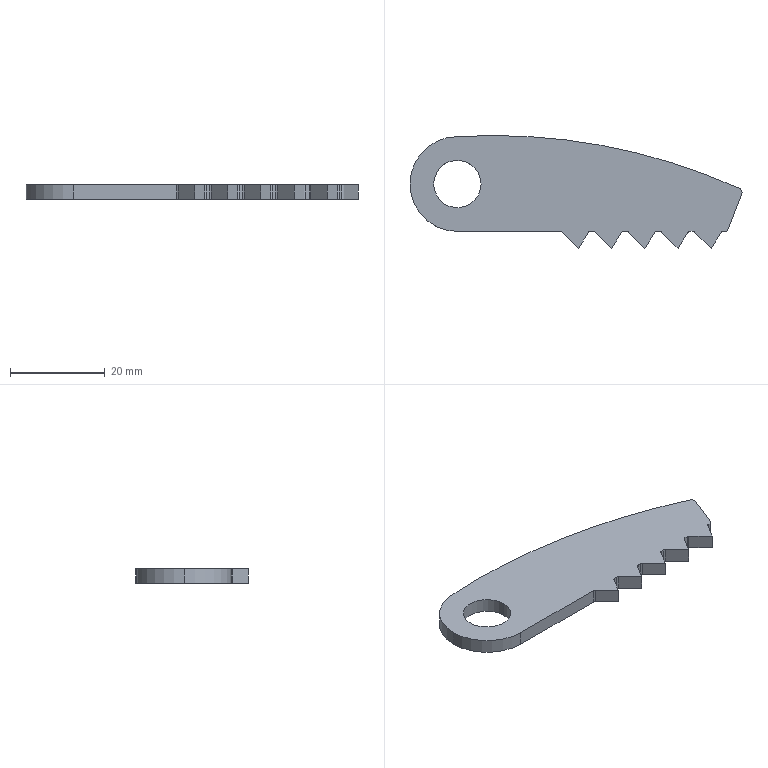Part | SolidWorks | features Extrusion 1, ICE 1 | 1 solid | 36 faces | box 70.059 x 23.839 x 3 mm | volume 3412 mm3 | plane 19 | cylinder 17 | commonest cylinder face diameters 1 x11 10 x2 20 x2 2 x1 252.737 x1
STEP:
#1=CARTESIAN_POINT('',(-5.,0.,0.));
#2=VERTEX_POINT('',#1);
#3=CARTESIAN_POINT('',(5.,0.,0.));
#4=VERTEX_POINT('',#3);
#5=CARTESIAN_POINT('',(0.,0.,0.));
#6=DIRECTION('',(0.,0.,1.));
#7=DIRECTION('',(1.,0.,0.));
#8=AXIS2_PLACEMENT_3D('',#5,#6,#7);
#9=CIRCLE('',#8,5.);
#10=EDGE_CURVE('',#2,#4,#9,.T.);
#11=ORIENTED_EDGE('',*,*,#10,.F.);
#12=CARTESIAN_POINT('',(-5.,0.,3.));
#13=VERTEX_POINT('',#12);
#14=CARTESIAN_POINT('',(-5.,0.,0.));
#15=DIRECTION('',(0.,0.,1.));
#16=VECTOR('',#15,1000.);
#17=LINE('',#14,#16);
#18=EDGE_CURVE('',#2,#13,#17,.T.);
#19=ORIENTED_EDGE('',*,*,#18,.T.);
#20=CARTESIAN_POINT('',(5.,0.,3.));
#21=VERTEX_POINT('',#20);
#22=CARTESIAN_POINT('',(0.,0.,3.));
#23=DIRECTION('',(0.,0.,1.));
#24=DIRECTION('',(1.,0.,0.));
#25=AXIS2_PLACEMENT_3D('',#22,#23,#24);
#26=CIRCLE('',#25,5.);
#27=EDGE_CURVE('',#13,#21,#26,.T.);
#28=ORIENTED_EDGE('',*,*,#27,.T.);
#29=CARTESIAN_POINT('',(5.,0.,0.));
#30=DIRECTION('',(0.,0.,1.));
#31=VECTOR('',#30,1000.);
#32=LINE('',#29,#31);
#33=EDGE_CURVE('',#4,#21,#32,.T.);
#34=ORIENTED_EDGE('',*,*,#33,.F.);
#35=EDGE_LOOP('',(#11,#19,#28,#34));
#36=FACE_OUTER_BOUND('',#35,.T.);
#37=CARTESIAN_POINT('',(0.,0.,0.));
#38=DIRECTION('',(0.,0.,1.));
#39=DIRECTION('',(1.,0.,0.));
#40=AXIS2_PLACEMENT_3D('',#37,#38,#39);
#41=CYLINDRICAL_SURFACE('',#40,5.);
#42=ADVANCED_FACE('',(#36),#41,.F.);
#43=CARTESIAN_POINT('',(-10.,0.,3.));
#44=VERTEX_POINT('',#43);
#45=CARTESIAN_POINT('',(0.,-10.,3.));
#46=VERTEX_POINT('',#45);
#47=CARTESIAN_POINT('',(0.,0.,3.));
#48=DIRECTION('',(0.,0.,1.));
#49=DIRECTION('',(1.,0.,0.));
#50=AXIS2_PLACEMENT_3D('',#47,#48,#49);
#51=CIRCLE('',#50,10.);
#52=EDGE_CURVE('',#44,#46,#51,.T.);
#53=ORIENTED_EDGE('',*,*,#52,.F.);
#54=CARTESIAN_POINT('',(-10.,0.,0.));
#55=VERTEX_POINT('',#54);
#56=CARTESIAN_POINT('',(-10.,0.,3.));
#57=DIRECTION('',(0.,0.,-1.));
#58=VECTOR('',#57,1000.);
#59=LINE('',#56,#58);
#60=EDGE_CURVE('',#44,#55,#59,.T.);
#61=ORIENTED_EDGE('',*,*,#60,.T.);
#62=CARTESIAN_POINT('',(0.,-10.,0.));
#63=VERTEX_POINT('',#62);
#64=CARTESIAN_POINT('',(0.,0.,0.));
#65=DIRECTION('',(0.,0.,1.));
#66=DIRECTION('',(1.,0.,0.));
#67=AXIS2_PLACEMENT_3D('',#64,#65,#66);
#68=CIRCLE('',#67,10.);
#69=EDGE_CURVE('',#55,#63,#68,.T.);
#70=ORIENTED_EDGE('',*,*,#69,.T.);
#71=CARTESIAN_POINT('',(0.,-10.,3.));
#72=DIRECTION('',(0.,0.,-1.));
#73=VECTOR('',#72,1000.);
#74=LINE('',#71,#73);
#75=EDGE_CURVE('',#46,#63,#74,.T.);
#76=ORIENTED_EDGE('',*,*,#75,.F.);
#77=EDGE_LOOP('',(#53,#61,#70,#76));
#78=FACE_OUTER_BOUND('',#77,.T.);
#79=CARTESIAN_POINT('',(0.,0.,3.));
#80=DIRECTION('',(0.,0.,-1.));
#81=DIRECTION('',(-1.,0.,0.));
#82=AXIS2_PLACEMENT_3D('',#79,#80,#81);
#83=CYLINDRICAL_SURFACE('',#82,10.);
#84=ADVANCED_FACE('',(#78),#83,.T.);
#85=ORIENTED_EDGE('',*,*,#60,.F.);
#86=CARTESIAN_POINT('',(-0.189,9.998,3.));
#87=VERTEX_POINT('',#86);
#88=CARTESIAN_POINT('',(0.,0.,3.));
#89=DIRECTION('',(0.,0.,1.));
#90=DIRECTION('',(1.,0.,0.));
#91=AXIS2_PLACEMENT_3D('',#88,#89,#90);
#92=CIRCLE('',#91,10.);
#93=EDGE_CURVE('',#87,#44,#92,.T.);
#94=ORIENTED_EDGE('',*,*,#93,.F.);
#95=CARTESIAN_POINT('',(-0.189,9.998,0.));
#96=VERTEX_POINT('',#95);
#97=CARTESIAN_POINT('',(-0.189,9.998,3.));
#98=DIRECTION('',(0.,0.,-1.));
#99=VECTOR('',#98,1000.);
#100=LINE('',#97,#99);
#101=EDGE_CURVE('',#87,#96,#100,.T.);
#102=ORIENTED_EDGE('',*,*,#101,.T.);
#103=CARTESIAN_POINT('',(0.,0.,0.));
#104=DIRECTION('',(0.,0.,1.));
#105=DIRECTION('',(1.,0.,0.));
#106=AXIS2_PLACEMENT_3D('',#103,#104,#105);
#107=CIRCLE('',#106,10.);
#108=EDGE_CURVE('',#96,#55,#107,.T.);
#109=ORIENTED_EDGE('',*,*,#108,.T.);
#110=EDGE_LOOP('',(#85,#94,#102,#109));
#111=FACE_OUTER_BOUND('',#110,.T.);
#112=CARTESIAN_POINT('',(0.,0.,3.));
#113=DIRECTION('',(0.,0.,-1.));
#114=DIRECTION('',(-1.,0.,0.));
#115=AXIS2_PLACEMENT_3D('',#112,#113,#114);
#116=CYLINDRICAL_SURFACE('',#115,10.);
#117=ADVANCED_FACE('',(#111),#116,.T.);
#118=CARTESIAN_POINT('',(21.748,-10.,0.));
#119=VERTEX_POINT('',#118);
#120=CARTESIAN_POINT('',(0.,-10.,0.));
#121=DIRECTION('',(1.,0.,0.));
#122=VECTOR('',#121,1000.);
#123=LINE('',#120,#122);
#124=EDGE_CURVE('',#63,#119,#123,.T.);
#125=ORIENTED_EDGE('',*,*,#124,.T.);
#126=CARTESIAN_POINT('',(21.748,-10.,3.));
#127=VERTEX_POINT('',#126);
#128=CARTESIAN_POINT('',(21.748,-10.,3.));
#129=DIRECTION('',(0.,0.,-1.));
#130=VECTOR('',#129,1000.);
#131=LINE('',#128,#130);
#132=EDGE_CURVE('',#127,#119,#131,.T.);
#133=ORIENTED_EDGE('',*,*,#132,.F.);
#134=CARTESIAN_POINT('',(0.,-10.,3.));
#135=DIRECTION('',(1.,0.,0.));
#136=VECTOR('',#135,1000.);
#137=LINE('',#134,#136);
#138=EDGE_CURVE('',#46,#127,#137,.T.);
#139=ORIENTED_EDGE('',*,*,#138,.F.);
#140=ORIENTED_EDGE('',*,*,#75,.T.);
#141=EDGE_LOOP('',(#125,#133,#139,#140));
#142=FACE_OUTER_BOUND('',#141,.T.);
#143=CARTESIAN_POINT('',(0.,-10.,3.));
#144=DIRECTION('',(0.,1.,0.));
#145=DIRECTION('',(0.,0.,1.));
#146=AXIS2_PLACEMENT_3D('',#143,#144,#145);
#147=PLANE('',#146);
#148=ADVANCED_FACE('',(#142),#147,.F.);
#149=CARTESIAN_POINT('',(22.101,-10.146,0.));
#150=VERTEX_POINT('',#149);
#151=CARTESIAN_POINT('',(21.748,-10.5,0.));
#152=DIRECTION('',(0.,0.,-1.));
#153=DIRECTION('',(1.,0.,0.));
#154=AXIS2_PLACEMENT_3D('',#151,#152,#153);
#155=CIRCLE('',#154,0.5);
#156=EDGE_CURVE('',#119,#150,#155,.T.);
#157=ORIENTED_EDGE('',*,*,#156,.T.);
#158=CARTESIAN_POINT('',(22.101,-10.146,3.));
#159=VERTEX_POINT('',#158);
#160=CARTESIAN_POINT('',(22.101,-10.146,3.));
#161=DIRECTION('',(0.,0.,-1.));
#162=VECTOR('',#161,1000.);
#163=LINE('',#160,#162);
#164=EDGE_CURVE('',#159,#150,#163,.T.);
#165=ORIENTED_EDGE('',*,*,#164,.F.);
#166=CARTESIAN_POINT('',(21.748,-10.5,3.));
#167=DIRECTION('',(0.,0.,-1.));
#168=DIRECTION('',(1.,0.,0.));
#169=AXIS2_PLACEMENT_3D('',#166,#167,#168);
#170=CIRCLE('',#169,0.5);
#171=EDGE_CURVE('',#127,#159,#170,.T.);
#172=ORIENTED_EDGE('',*,*,#171,.F.);
#173=ORIENTED_EDGE('',*,*,#132,.T.);
#174=EDGE_LOOP('',(#157,#165,#172,#173));
#175=FACE_OUTER_BOUND('',#174,.T.);
#176=CARTESIAN_POINT('',(21.748,-10.5,3.));
#177=DIRECTION('',(0.,0.,-1.));
#178=DIRECTION('',(-1.,0.,0.));
#179=AXIS2_PLACEMENT_3D('',#176,#177,#178);
#180=CYLINDRICAL_SURFACE('',#179,0.5);
#181=ADVANCED_FACE('',(#175),#180,.F.);
#182=CARTESIAN_POINT('',(25.559,-13.604,0.));
#183=VERTEX_POINT('',#182);
#184=CARTESIAN_POINT('',(22.101,-10.146,0.));
#185=DIRECTION('',(0.7071,-0.7071,0.));
#186=VECTOR('',#185,1000.);
#187=LINE('',#184,#186);
#188=EDGE_CURVE('',#150,#183,#187,.T.);
#189=ORIENTED_EDGE('',*,*,#188,.T.);
#190=CARTESIAN_POINT('',(25.559,-13.604,3.));
#191=VERTEX_POINT('',#190);
#192=CARTESIAN_POINT('',(25.559,-13.604,3.));
#193=DIRECTION('',(0.,0.,-1.));
#194=VECTOR('',#193,1000.);
#195=LINE('',#192,#194);
#196=EDGE_CURVE('',#191,#183,#195,.T.);
#197=ORIENTED_EDGE('',*,*,#196,.F.);
#198=CARTESIAN_POINT('',(22.101,-10.146,3.));
#199=DIRECTION('',(0.7071,-0.7071,0.));
#200=VECTOR('',#199,1000.);
#201=LINE('',#198,#200);
#202=EDGE_CURVE('',#159,#191,#201,.T.);
#203=ORIENTED_EDGE('',*,*,#202,.F.);
#204=ORIENTED_EDGE('',*,*,#164,.T.);
#205=EDGE_LOOP('',(#189,#197,#203,#204));
#206=FACE_OUTER_BOUND('',#205,.T.);
#207=CARTESIAN_POINT('',(22.101,-10.146,3.));
#208=DIRECTION('',(0.7071,0.7071,0.));
#209=DIRECTION('',(-0.7071,0.7071,0.));
#210=AXIS2_PLACEMENT_3D('',#207,#208,#209);
#211=PLANE('',#210);
#212=ADVANCED_FACE('',(#206),#211,.F.);
#213=CARTESIAN_POINT('',(27.631,-10.238,0.));
#214=VERTEX_POINT('',#213);
#215=CARTESIAN_POINT('',(25.559,-13.604,0.));
#216=DIRECTION('',(0.5242,0.8516,0.));
#217=VECTOR('',#216,1000.);
#218=LINE('',#215,#217);
#219=EDGE_CURVE('',#183,#214,#218,.T.);
#220=ORIENTED_EDGE('',*,*,#219,.T.);
#221=CARTESIAN_POINT('',(27.631,-10.238,3.));
#222=VERTEX_POINT('',#221);
#223=CARTESIAN_POINT('',(27.631,-10.238,3.));
#224=DIRECTION('',(0.,0.,-1.));
#225=VECTOR('',#224,1000.);
#226=LINE('',#223,#225);
#227=EDGE_CURVE('',#222,#214,#226,.T.);
#228=ORIENTED_EDGE('',*,*,#227,.F.);
#229=CARTESIAN_POINT('',(25.559,-13.604,3.));
#230=DIRECTION('',(0.5242,0.8516,0.));
#231=VECTOR('',#230,1000.);
#232=LINE('',#229,#231);
#233=EDGE_CURVE('',#191,#222,#232,.T.);
#234=ORIENTED_EDGE('',*,*,#233,.F.);
#235=ORIENTED_EDGE('',*,*,#196,.T.);
#236=EDGE_LOOP('',(#220,#228,#234,#235));
#237=FACE_OUTER_BOUND('',#236,.T.);
#238=CARTESIAN_POINT('',(25.559,-13.604,3.));
#239=DIRECTION('',(-0.8516,0.5242,0.));
#240=DIRECTION('',(-0.5242,-0.8516,0.));
#241=AXIS2_PLACEMENT_3D('',#238,#239,#240);
#242=PLANE('',#241);
#243=ADVANCED_FACE('',(#237),#242,.F.);
#244=CARTESIAN_POINT('',(28.056,-10.,0.));
#245=VERTEX_POINT('',#244);
#246=CARTESIAN_POINT('',(28.056,-10.5,0.));
#247=DIRECTION('',(0.,0.,-1.));
#248=DIRECTION('',(1.,0.,0.));
#249=AXIS2_PLACEMENT_3D('',#246,#247,#248);
#250=CIRCLE('',#249,0.5);
#251=EDGE_CURVE('',#214,#245,#250,.T.);
#252=ORIENTED_EDGE('',*,*,#251,.T.);
#253=CARTESIAN_POINT('',(28.056,-10.,3.));
#254=VERTEX_POINT('',#253);
#255=CARTESIAN_POINT('',(28.056,-10.,3.));
#256=DIRECTION('',(0.,0.,-1.));
#257=VECTOR('',#256,1000.);
#258=LINE('',#255,#257);
#259=EDGE_CURVE('',#254,#245,#258,.T.);
#260=ORIENTED_EDGE('',*,*,#259,.F.);
#261=CARTESIAN_POINT('',(28.056,-10.5,3.));
#262=DIRECTION('',(0.,0.,-1.));
#263=DIRECTION('',(1.,0.,0.));
#264=AXIS2_PLACEMENT_3D('',#261,#262,#263);
#265=CIRCLE('',#264,0.5);
#266=EDGE_CURVE('',#222,#254,#265,.T.);
#267=ORIENTED_EDGE('',*,*,#266,.F.);
#268=ORIENTED_EDGE('',*,*,#227,.T.);
#269=EDGE_LOOP('',(#252,#260,#267,#268));
#270=FACE_OUTER_BOUND('',#269,.T.);
#271=CARTESIAN_POINT('',(28.056,-10.5,3.));
#272=DIRECTION('',(0.,0.,-1.));
#273=DIRECTION('',(-1.,0.,0.));
#274=AXIS2_PLACEMENT_3D('',#271,#272,#273);
#275=CYLINDRICAL_SURFACE('',#274,0.5);
#276=ADVANCED_FACE('',(#270),#275,.F.);
#277=CARTESIAN_POINT('',(28.748,-10.,0.));
#278=VERTEX_POINT('',#277);
#279=CARTESIAN_POINT('',(28.056,-10.,0.));
#280=DIRECTION('',(1.,0.,0.));
#281=VECTOR('',#280,1000.);
#282=LINE('',#279,#281);
#283=EDGE_CURVE('',#245,#278,#282,.T.);
#284=ORIENTED_EDGE('',*,*,#283,.T.);
#285=CARTESIAN_POINT('',(28.748,-10.,3.));
#286=VERTEX_POINT('',#285);
#287=CARTESIAN_POINT('',(28.748,-10.,3.));
#288=DIRECTION('',(0.,0.,-1.));
#289=VECTOR('',#288,1000.);
#290=LINE('',#287,#289);
#291=EDGE_CURVE('',#286,#278,#290,.T.);
#292=ORIENTED_EDGE('',*,*,#291,.F.);
#293=CARTESIAN_POINT('',(28.056,-10.,3.));
#294=DIRECTION('',(1.,0.,0.));
#295=VECTOR('',#294,1000.);
#296=LINE('',#293,#295);
#297=EDGE_CURVE('',#254,#286,#296,.T.);
#298=ORIENTED_EDGE('',*,*,#297,.F.);
#299=ORIENTED_EDGE('',*,*,#259,.T.);
#300=EDGE_LOOP('',(#284,#292,#298,#299));
#301=FACE_OUTER_BOUND('',#300,.T.);
#302=CARTESIAN_POINT('',(28.056,-10.,3.));
#303=DIRECTION('',(0.,1.,0.));
#304=DIRECTION('',(0.,0.,1.));
#305=AXIS2_PLACEMENT_3D('',#302,#303,#304);
#306=PLANE('',#305);
#307=ADVANCED_FACE('',(#301),#306,.F.);
#308=CARTESIAN_POINT('',(29.101,-10.146,0.));
#309=VERTEX_POINT('',#308);
#310=CARTESIAN_POINT('',(28.748,-10.5,0.));
#311=DIRECTION('',(0.,0.,-1.));
#312=DIRECTION('',(-1.,0.,0.));
#313=AXIS2_PLACEMENT_3D('',#310,#311,#312);
#314=CIRCLE('',#313,0.5);
#315=EDGE_CURVE('',#278,#309,#314,.T.);
#316=ORIENTED_EDGE('',*,*,#315,.T.);
#317=CARTESIAN_POINT('',(29.101,-10.146,3.));
#318=VERTEX_POINT('',#317);
#319=CARTESIAN_POINT('',(29.101,-10.146,3.));
#320=DIRECTION('',(0.,0.,-1.));
#321=VECTOR('',#320,1000.);
#322=LINE('',#319,#321);
#323=EDGE_CURVE('',#318,#309,#322,.T.);
#324=ORIENTED_EDGE('',*,*,#323,.F.);
#325=CARTESIAN_POINT('',(28.748,-10.5,3.));
#326=DIRECTION('',(0.,0.,-1.));
#327=DIRECTION('',(-1.,0.,0.));
#328=AXIS2_PLACEMENT_3D('',#325,#326,#327);
#329=CIRCLE('',#328,0.5);
#330=EDGE_CURVE('',#286,#318,#329,.T.);
#331=ORIENTED_EDGE('',*,*,#330,.F.);
#332=ORIENTED_EDGE('',*,*,#291,.T.);
#333=EDGE_LOOP('',(#316,#324,#331,#332));
#334=FACE_OUTER_BOUND('',#333,.T.);
#335=CARTESIAN_POINT('',(28.748,-10.5,3.));
#336=DIRECTION('',(0.,0.,-1.));
#337=DIRECTION('',(-1.,0.,0.));
#338=AXIS2_PLACEMENT_3D('',#335,#336,#337);
#339=CYLINDRICAL_SURFACE('',#338,0.5);
#340=ADVANCED_FACE('',(#334),#339,.F.);
#341=CARTESIAN_POINT('',(32.559,-13.604,0.));
#342=VERTEX_POINT('',#341);
#343=CARTESIAN_POINT('',(29.101,-10.146,0.));
#344=DIRECTION('',(0.7071,-0.7071,0.));
#345=VECTOR('',#344,1000.);
#346=LINE('',#343,#345);
#347=EDGE_CURVE('',#309,#342,#346,.T.);
#348=ORIENTED_EDGE('',*,*,#347,.T.);
#349=CARTESIAN_POINT('',(32.559,-13.604,3.));
#350=VERTEX_POINT('',#349);
#351=CARTESIAN_POINT('',(32.559,-13.604,3.));
#352=DIRECTION('',(0.,0.,-1.));
#353=VECTOR('',#352,1000.);
#354=LINE('',#351,#353);
#355=EDGE_CURVE('',#350,#342,#354,.T.);
#356=ORIENTED_EDGE('',*,*,#355,.F.);
#357=CARTESIAN_POINT('',(29.101,-10.146,3.));
#358=DIRECTION('',(0.7071,-0.7071,0.));
#359=VECTOR('',#358,1000.);
#360=LINE('',#357,#359);
#361=EDGE_CURVE('',#318,#350,#360,.T.);
#362=ORIENTED_EDGE('',*,*,#361,.F.);
#363=ORIENTED_EDGE('',*,*,#323,.T.);
#364=EDGE_LOOP('',(#348,#356,#362,#363));
#365=FACE_OUTER_BOUND('',#364,.T.);
#366=CARTESIAN_POINT('',(29.101,-10.146,3.));
#367=DIRECTION('',(0.7071,0.7071,0.));
#368=DIRECTION('',(-0.7071,0.7071,0.));
#369=AXIS2_PLACEMENT_3D('',#366,#367,#368);
#370=PLANE('',#369);
#371=ADVANCED_FACE('',(#365),#370,.F.);
#372=CARTESIAN_POINT('',(34.631,-10.238,0.));
#373=VERTEX_POINT('',#372);
#374=CARTESIAN_POINT('',(32.559,-13.604,0.));
#375=DIRECTION('',(0.5242,0.8516,0.));
#376=VECTOR('',#375,1000.);
#377=LINE('',#374,#376);
#378=EDGE_CURVE('',#342,#373,#377,.T.);
#379=ORIENTED_EDGE('',*,*,#378,.T.);
#380=CARTESIAN_POINT('',(34.631,-10.238,3.));
#381=VERTEX_POINT('',#380);
#382=CARTESIAN_POINT('',(34.631,-10.238,3.));
#383=DIRECTION('',(0.,0.,-1.));
#384=VECTOR('',#383,1000.);
#385=LINE('',#382,#384);
#386=EDGE_CURVE('',#381,#373,#385,.T.);
#387=ORIENTED_EDGE('',*,*,#386,.F.);
#388=CARTESIAN_POINT('',(32.559,-13.604,3.));
#389=DIRECTION('',(0.5242,0.8516,0.));
#390=VECTOR('',#389,1000.);
#391=LINE('',#388,#390);
#392=EDGE_CURVE('',#350,#381,#391,.T.);
#393=ORIENTED_EDGE('',*,*,#392,.F.);
#394=ORIENTED_EDGE('',*,*,#355,.T.);
#395=EDGE_LOOP('',(#379,#387,#393,#394));
#396=FACE_OUTER_BOUND('',#395,.T.);
#397=CARTESIAN_POINT('',(32.559,-13.604,3.));
#398=DIRECTION('',(-0.8516,0.5242,0.));
#399=DIRECTION('',(-0.5242,-0.8516,0.));
#400=AXIS2_PLACEMENT_3D('',#397,#398,#399);
#401=PLANE('',#400);
#402=ADVANCED_FACE('',(#396),#401,.F.);
#403=CARTESIAN_POINT('',(35.056,-10.,0.));
#404=VERTEX_POINT('',#403);
#405=CARTESIAN_POINT('',(35.056,-10.5,0.));
#406=DIRECTION('',(0.,0.,-1.));
#407=DIRECTION('',(1.,0.,0.));
#408=AXIS2_PLACEMENT_3D('',#405,#406,#407);
#409=CIRCLE('',#408,0.5);
#410=EDGE_CURVE('',#373,#404,#409,.T.);
#411=ORIENTED_EDGE('',*,*,#410,.T.);
#412=CARTESIAN_POINT('',(35.056,-10.,3.));
#413=VERTEX_POINT('',#412);
#414=CARTESIAN_POINT('',(35.056,-10.,3.));
#415=DIRECTION('',(0.,0.,-1.));
#416=VECTOR('',#415,1000.);
#417=LINE('',#414,#416);
#418=EDGE_CURVE('',#413,#404,#417,.T.);
#419=ORIENTED_EDGE('',*,*,#418,.F.);
#420=CARTESIAN_POINT('',(35.056,-10.5,3.));
#421=DIRECTION('',(0.,0.,-1.));
#422=DIRECTION('',(1.,0.,0.));
#423=AXIS2_PLACEMENT_3D('',#420,#421,#422);
#424=CIRCLE('',#423,0.5);
#425=EDGE_CURVE('',#381,#413,#424,.T.);
#426=ORIENTED_EDGE('',*,*,#425,.F.);
#427=ORIENTED_EDGE('',*,*,#386,.T.);
#428=EDGE_LOOP('',(#411,#419,#426,#427));
#429=FACE_OUTER_BOUND('',#428,.T.);
#430=CARTESIAN_POINT('',(35.056,-10.5,3.));
#431=DIRECTION('',(0.,0.,-1.));
#432=DIRECTION('',(-1.,0.,0.));
#433=AXIS2_PLACEMENT_3D('',#430,#431,#432);
#434=CYLINDRICAL_SURFACE('',#433,0.5);
#435=ADVANCED_FACE('',(#429),#434,.F.);
#436=CARTESIAN_POINT('',(35.748,-10.,0.));
#437=VERTEX_POINT('',#436);
#438=CARTESIAN_POINT('',(35.056,-10.,0.));
#439=DIRECTION('',(1.,0.,0.));
#440=VECTOR('',#439,1000.);
#441=LINE('',#438,#440);
#442=EDGE_CURVE('',#404,#437,#441,.T.);
#443=ORIENTED_EDGE('',*,*,#442,.T.);
#444=CARTESIAN_POINT('',(35.748,-10.,3.));
#445=VERTEX_POINT('',#444);
#446=CARTESIAN_POINT('',(35.748,-10.,3.));
#447=DIRECTION('',(0.,0.,-1.));
#448=VECTOR('',#447,1000.);
#449=LINE('',#446,#448);
#450=EDGE_CURVE('',#445,#437,#449,.T.);
#451=ORIENTED_EDGE('',*,*,#450,.F.);
#452=CARTESIAN_POINT('',(35.056,-10.,3.));
#453=DIRECTION('',(1.,0.,0.));
#454=VECTOR('',#453,1000.);
#455=LINE('',#452,#454);
#456=EDGE_CURVE('',#413,#445,#455,.T.);
#457=ORIENTED_EDGE('',*,*,#456,.F.);
#458=ORIENTED_EDGE('',*,*,#418,.T.);
#459=EDGE_LOOP('',(#443,#451,#457,#458));
#460=FACE_OUTER_BOUND('',#459,.T.);
#461=CARTESIAN_POINT('',(35.056,-10.,3.));
#462=DIRECTION('',(0.,1.,0.));
#463=DIRECTION('',(0.,0.,1.));
#464=AXIS2_PLACEMENT_3D('',#461,#462,#463);
#465=PLANE('',#464);
#466=ADVANCED_FACE('',(#460),#465,.F.);
#467=CARTESIAN_POINT('',(36.101,-10.146,0.));
#468=VERTEX_POINT('',#467);
#469=CARTESIAN_POINT('',(35.748,-10.5,0.));
#470=DIRECTION('',(0.,0.,-1.));
#471=DIRECTION('',(-1.,0.,0.));
#472=AXIS2_PLACEMENT_3D('',#469,#470,#471);
#473=CIRCLE('',#472,0.5);
#474=EDGE_CURVE('',#437,#468,#473,.T.);
#475=ORIENTED_EDGE('',*,*,#474,.T.);
#476=CARTESIAN_POINT('',(36.101,-10.146,3.));
#477=VERTEX_POINT('',#476);
#478=CARTESIAN_POINT('',(36.101,-10.146,3.));
#479=DIRECTION('',(0.,0.,-1.));
#480=VECTOR('',#479,1000.);
#481=LINE('',#478,#480);
#482=EDGE_CURVE('',#477,#468,#481,.T.);
#483=ORIENTED_EDGE('',*,*,#482,.F.);
#484=CARTESIAN_POINT('',(35.748,-10.5,3.));
#485=DIRECTION('',(0.,0.,-1.));
#486=DIRECTION('',(-1.,0.,0.));
#487=AXIS2_PLACEMENT_3D('',#484,#485,#486);
#488=CIRCLE('',#487,0.5);
#489=EDGE_CURVE('',#445,#477,#488,.T.);
#490=ORIENTED_EDGE('',*,*,#489,.F.);
#491=ORIENTED_EDGE('',*,*,#450,.T.);
#492=EDGE_LOOP('',(#475,#483,#490,#491));
#493=FACE_OUTER_BOUND('',#492,.T.);
#494=CARTESIAN_POINT('',(35.748,-10.5,3.));
#495=DIRECTION('',(0.,0.,-1.));
#496=DIRECTION('',(-1.,0.,0.));
#497=AXIS2_PLACEMENT_3D('',#494,#495,#496);
#498=CYLINDRICAL_SURFACE('',#497,0.5);
#499=ADVANCED_FACE('',(#493),#498,.F.);
#500=CARTESIAN_POINT('',(39.559,-13.604,0.));
#501=VERTEX_POINT('',#500);
#502=CARTESIAN_POINT('',(36.101,-10.146,0.));
#503=DIRECTION('',(0.7071,-0.7071,0.));
#504=VECTOR('',#503,1000.);
#505=LINE('',#502,#504);
#506=EDGE_CURVE('',#468,#501,#505,.T.);
#507=ORIENTED_EDGE('',*,*,#506,.T.);
#508=CARTESIAN_POINT('',(39.559,-13.604,3.));
#509=VERTEX_POINT('',#508);
#510=CARTESIAN_POINT('',(39.559,-13.604,3.));
#511=DIRECTION('',(0.,0.,-1.));
#512=VECTOR('',#511,1000.);
#513=LINE('',#510,#512);
#514=EDGE_CURVE('',#509,#501,#513,.T.);
#515=ORIENTED_EDGE('',*,*,#514,.F.);
#516=CARTESIAN_POINT('',(36.101,-10.146,3.));
#517=DIRECTION('',(0.7071,-0.7071,0.));
#518=VECTOR('',#517,1000.);
#519=LINE('',#516,#518);
#520=EDGE_CURVE('',#477,#509,#519,.T.);
#521=ORIENTED_EDGE('',*,*,#520,.F.);
#522=ORIENTED_EDGE('',*,*,#482,.T.);
#523=EDGE_LOOP('',(#507,#515,#521,#522));
#524=FACE_OUTER_BOUND('',#523,.T.);
#525=CARTESIAN_POINT('',(36.101,-10.146,3.));
#526=DIRECTION('',(0.7071,0.7071,0.));
#527=DIRECTION('',(-0.7071,0.7071,0.));
#528=AXIS2_PLACEMENT_3D('',#525,#526,#527);
#529=PLANE('',#528);
#530=ADVANCED_FACE('',(#524),#529,.F.);
#531=CARTESIAN_POINT('',(41.631,-10.238,0.));
#532=VERTEX_POINT('',#531);
#533=CARTESIAN_POINT('',(39.559,-13.604,0.));
#534=DIRECTION('',(0.5242,0.8516,0.));
#535=VECTOR('',#534,1000.);
#536=LINE('',#533,#535);
#537=EDGE_CURVE('',#501,#532,#536,.T.);
#538=ORIENTED_EDGE('',*,*,#537,.T.);
#539=CARTESIAN_POINT('',(41.631,-10.238,3.));
#540=VERTEX_POINT('',#539);
#541=CARTESIAN_POINT('',(41.631,-10.238,3.));
#542=DIRECTION('',(0.,0.,-1.));
#543=VECTOR('',#542,1000.);
#544=LINE('',#541,#543);
#545=EDGE_CURVE('',#540,#532,#544,.T.);
#546=ORIENTED_EDGE('',*,*,#545,.F.);
#547=CARTESIAN_POINT('',(39.559,-13.604,3.));
#548=DIRECTION('',(0.5242,0.8516,0.));
#549=VECTOR('',#548,1000.);
#550=LINE('',#547,#549);
#551=EDGE_CURVE('',#509,#540,#550,.T.);
#552=ORIENTED_EDGE('',*,*,#551,.F.);
#553=ORIENTED_EDGE('',*,*,#514,.T.);
#554=EDGE_LOOP('',(#538,#546,#552,#553));
#555=FACE_OUTER_BOUND('',#554,.T.);
#556=CARTESIAN_POINT('',(39.559,-13.604,3.));
#557=DIRECTION('',(-0.8516,0.5242,0.));
#558=DIRECTION('',(-0.5242,-0.8516,0.));
#559=AXIS2_PLACEMENT_3D('',#556,#557,#558);
#560=PLANE('',#559);
#561=ADVANCED_FACE('',(#555),#560,.F.);
#562=CARTESIAN_POINT('',(42.056,-10.,0.));
#563=VERTEX_POINT('',#562);
#564=CARTESIAN_POINT('',(42.056,-10.5,0.));
#565=DIRECTION('',(0.,0.,-1.));
#566=DIRECTION('',(1.,0.,0.));
#567=AXIS2_PLACEMENT_3D('',#564,#565,#566);
#568=CIRCLE('',#567,0.5);
#569=EDGE_CURVE('',#532,#563,#568,.T.);
#570=ORIENTED_EDGE('',*,*,#569,.T.);
#571=CARTESIAN_POINT('',(42.056,-10.,3.));
#572=VERTEX_POINT('',#571);
#573=CARTESIAN_POINT('',(42.056,-10.,3.));
#574=DIRECTION('',(0.,0.,-1.));
#575=VECTOR('',#574,1000.);
#576=LINE('',#573,#575);
#577=EDGE_CURVE('',#572,#563,#576,.T.);
#578=ORIENTED_EDGE('',*,*,#577,.F.);
#579=CARTESIAN_POINT('',(42.056,-10.5,3.));
#580=DIRECTION('',(0.,0.,-1.));
#581=DIRECTION('',(1.,0.,0.));
#582=AXIS2_PLACEMENT_3D('',#579,#580,#581);
#583=CIRCLE('',#582,0.5);
#584=EDGE_CURVE('',#540,#572,#583,.T.);
#585=ORIENTED_EDGE('',*,*,#584,.F.);
#586=ORIENTED_EDGE('',*,*,#545,.T.);
#587=EDGE_LOOP('',(#570,#578,#585,#586));
#588=FACE_OUTER_BOUND('',#587,.T.);
#589=CARTESIAN_POINT('',(42.056,-10.5,3.));
#590=DIRECTION('',(0.,0.,-1.));
#591=DIRECTION('',(-1.,0.,0.));
#592=AXIS2_PLACEMENT_3D('',#589,#590,#591);
#593=CYLINDRICAL_SURFACE('',#592,0.5);
#594=ADVANCED_FACE('',(#588),#593,.F.);
#595=CARTESIAN_POINT('',(42.748,-10.,0.));
#596=VERTEX_POINT('',#595);
#597=CARTESIAN_POINT('',(42.056,-10.,0.));
#598=DIRECTION('',(1.,0.,0.));
#599=VECTOR('',#598,1000.);
#600=LINE('',#597,#599);
#601=EDGE_CURVE('',#563,#596,#600,.T.);
#602=ORIENTED_EDGE('',*,*,#601,.T.);
#603=CARTESIAN_POINT('',(42.748,-10.,3.));
#604=VERTEX_POINT('',#603);
#605=CARTESIAN_POINT('',(42.748,-10.,3.));
#606=DIRECTION('',(0.,0.,-1.));
#607=VECTOR('',#606,1000.);
#608=LINE('',#605,#607);
#609=EDGE_CURVE('',#604,#596,#608,.T.);
#610=ORIENTED_EDGE('',*,*,#609,.F.);
#611=CARTESIAN_POINT('',(42.056,-10.,3.));
#612=DIRECTION('',(1.,0.,0.));
#613=VECTOR('',#612,1000.);
#614=LINE('',#611,#613);
#615=EDGE_CURVE('',#572,#604,#614,.T.);
#616=ORIENTED_EDGE('',*,*,#615,.F.);
#617=ORIENTED_EDGE('',*,*,#577,.T.);
#618=EDGE_LOOP('',(#602,#610,#616,#617));
#619=FACE_OUTER_BOUND('',#618,.T.);
#620=CARTESIAN_POINT('',(42.056,-10.,3.));
#621=DIRECTION('',(0.,1.,0.));
#622=DIRECTION('',(0.,0.,1.));
#623=AXIS2_PLACEMENT_3D('',#620,#621,#622);
#624=PLANE('',#623);
#625=ADVANCED_FACE('',(#619),#624,.F.);
#626=CARTESIAN_POINT('',(43.101,-10.146,0.));
#627=VERTEX_POINT('',#626);
#628=CARTESIAN_POINT('',(42.748,-10.5,0.));
#629=DIRECTION('',(0.,0.,-1.));
#630=DIRECTION('',(-1.,0.,0.));
#631=AXIS2_PLACEMENT_3D('',#628,#629,#630);
#632=CIRCLE('',#631,0.5);
#633=EDGE_CURVE('',#596,#627,#632,.T.);
#634=ORIENTED_EDGE('',*,*,#633,.T.);
#635=CARTESIAN_POINT('',(43.101,-10.146,3.));
#636=VERTEX_POINT('',#635);
#637=CARTESIAN_POINT('',(43.101,-10.146,3.));
#638=DIRECTION('',(0.,0.,-1.));
#639=VECTOR('',#638,1000.);
#640=LINE('',#637,#639);
#641=EDGE_CURVE('',#636,#627,#640,.T.);
#642=ORIENTED_EDGE('',*,*,#641,.F.);
#643=CARTESIAN_POINT('',(42.748,-10.5,3.));
#644=DIRECTION('',(0.,0.,-1.));
#645=DIRECTION('',(-1.,0.,0.));
#646=AXIS2_PLACEMENT_3D('',#643,#644,#645);
#647=CIRCLE('',#646,0.5);
#648=EDGE_CURVE('',#604,#636,#647,.T.);
#649=ORIENTED_EDGE('',*,*,#648,.F.);
#650=ORIENTED_EDGE('',*,*,#609,.T.);
#651=EDGE_LOOP('',(#634,#642,#649,#650));
#652=FACE_OUTER_BOUND('',#651,.T.);
#653=CARTESIAN_POINT('',(42.748,-10.5,3.));
#654=DIRECTION('',(0.,0.,-1.));
#655=DIRECTION('',(-1.,0.,0.));
#656=AXIS2_PLACEMENT_3D('',#653,#654,#655);
#657=CYLINDRICAL_SURFACE('',#656,0.5);
#658=ADVANCED_FACE('',(#652),#657,.F.);
#659=CARTESIAN_POINT('',(46.559,-13.604,0.));
#660=VERTEX_POINT('',#659);
#661=CARTESIAN_POINT('',(43.101,-10.146,0.));
#662=DIRECTION('',(0.7071,-0.7071,0.));
#663=VECTOR('',#662,1000.);
#664=LINE('',#661,#663);
#665=EDGE_CURVE('',#627,#660,#664,.T.);
#666=ORIENTED_EDGE('',*,*,#665,.T.);
#667=CARTESIAN_POINT('',(46.559,-13.604,3.));
#668=VERTEX_POINT('',#667);
#669=CARTESIAN_POINT('',(46.559,-13.604,3.));
#670=DIRECTION('',(0.,0.,-1.));
#671=VECTOR('',#670,1000.);
#672=LINE('',#669,#671);
#673=EDGE_CURVE('',#668,#660,#672,.T.);
#674=ORIENTED_EDGE('',*,*,#673,.F.);
#675=CARTESIAN_POINT('',(43.101,-10.146,3.));
#676=DIRECTION('',(0.7071,-0.7071,0.));
#677=VECTOR('',#676,1000.);
#678=LINE('',#675,#677);
#679=EDGE_CURVE('',#636,#668,#678,.T.);
#680=ORIENTED_EDGE('',*,*,#679,.F.);
#681=ORIENTED_EDGE('',*,*,#641,.T.);
#682=EDGE_LOOP('',(#666,#674,#680,#681));
#683=FACE_OUTER_BOUND('',#682,.T.);
#684=CARTESIAN_POINT('',(43.101,-10.146,3.));
#685=DIRECTION('',(0.7071,0.7071,0.));
#686=DIRECTION('',(-0.7071,0.7071,0.));
#687=AXIS2_PLACEMENT_3D('',#684,#685,#686);
#688=PLANE('',#687);
#689=ADVANCED_FACE('',(#683),#688,.F.);
#690=CARTESIAN_POINT('',(48.631,-10.238,0.));
#691=VERTEX_POINT('',#690);
#692=CARTESIAN_POINT('',(46.559,-13.604,0.));
#693=DIRECTION('',(0.5242,0.8516,0.));
#694=VECTOR('',#693,1000.);
#695=LINE('',#692,#694);
#696=EDGE_CURVE('',#660,#691,#695,.T.);
#697=ORIENTED_EDGE('',*,*,#696,.T.);
#698=CARTESIAN_POINT('',(48.631,-10.238,3.));
#699=VERTEX_POINT('',#698);
#700=CARTESIAN_POINT('',(48.631,-10.238,3.));
#701=DIRECTION('',(0.,0.,-1.));
#702=VECTOR('',#701,1000.);
#703=LINE('',#700,#702);
#704=EDGE_CURVE('',#699,#691,#703,.T.);
#705=ORIENTED_EDGE('',*,*,#704,.F.);
#706=CARTESIAN_POINT('',(46.559,-13.604,3.));
#707=DIRECTION('',(0.5242,0.8516,0.));
#708=VECTOR('',#707,1000.);
#709=LINE('',#706,#708);
#710=EDGE_CURVE('',#668,#699,#709,.T.);
#711=ORIENTED_EDGE('',*,*,#710,.F.);
#712=ORIENTED_EDGE('',*,*,#673,.T.);
#713=EDGE_LOOP('',(#697,#705,#711,#712));
#714=FACE_OUTER_BOUND('',#713,.T.);
#715=CARTESIAN_POINT('',(46.559,-13.604,3.));
#716=DIRECTION('',(-0.8516,0.5242,0.));
#717=DIRECTION('',(-0.5242,-0.8516,0.));
#718=AXIS2_PLACEMENT_3D('',#715,#716,#717);
#719=PLANE('',#718);
#720=ADVANCED_FACE('',(#714),#719,.F.);
#721=CARTESIAN_POINT('',(49.056,-10.,0.));
#722=VERTEX_POINT('',#721);
#723=CARTESIAN_POINT('',(49.056,-10.5,0.));
#724=DIRECTION('',(0.,0.,-1.));
#725=DIRECTION('',(1.,0.,0.));
#726=AXIS2_PLACEMENT_3D('',#723,#724,#725);
#727=CIRCLE('',#726,0.5);
#728=EDGE_CURVE('',#691,#722,#727,.T.);
#729=ORIENTED_EDGE('',*,*,#728,.T.);
#730=CARTESIAN_POINT('',(49.056,-10.,3.));
#731=VERTEX_POINT('',#730);
#732=CARTESIAN_POINT('',(49.056,-10.,3.));
#733=DIRECTION('',(0.,0.,-1.));
#734=VECTOR('',#733,1000.);
#735=LINE('',#732,#734);
#736=EDGE_CURVE('',#731,#722,#735,.T.);
#737=ORIENTED_EDGE('',*,*,#736,.F.);
#738=CARTESIAN_POINT('',(49.056,-10.5,3.));
#739=DIRECTION('',(0.,0.,-1.));
#740=DIRECTION('',(1.,0.,0.));
#741=AXIS2_PLACEMENT_3D('',#738,#739,#740);
#742=CIRCLE('',#741,0.5);
#743=EDGE_CURVE('',#699,#731,#742,.T.);
#744=ORIENTED_EDGE('',*,*,#743,.F.);
#745=ORIENTED_EDGE('',*,*,#704,.T.);
#746=EDGE_LOOP('',(#729,#737,#744,#745));
#747=FACE_OUTER_BOUND('',#746,.T.);
#748=CARTESIAN_POINT('',(49.056,-10.5,3.));
#749=DIRECTION('',(0.,0.,-1.));
#750=DIRECTION('',(-1.,0.,0.));
#751=AXIS2_PLACEMENT_3D('',#748,#749,#750);
#752=CYLINDRICAL_SURFACE('',#751,0.5);
#753=ADVANCED_FACE('',(#747),#752,.F.);
#754=CARTESIAN_POINT('',(49.748,-10.,0.));
#755=VERTEX_POINT('',#754);
#756=CARTESIAN_POINT('',(49.056,-10.,0.));
#757=DIRECTION('',(1.,0.,0.));
#758=VECTOR('',#757,1000.);
#759=LINE('',#756,#758);
#760=EDGE_CURVE('',#722,#755,#759,.T.);
#761=ORIENTED_EDGE('',*,*,#760,.T.);
#762=CARTESIAN_POINT('',(49.748,-10.,3.));
#763=VERTEX_POINT('',#762);
#764=CARTESIAN_POINT('',(49.748,-10.,3.));
#765=DIRECTION('',(0.,0.,-1.));
#766=VECTOR('',#765,1000.);
#767=LINE('',#764,#766);
#768=EDGE_CURVE('',#763,#755,#767,.T.);
#769=ORIENTED_EDGE('',*,*,#768,.F.);
#770=CARTESIAN_POINT('',(49.056,-10.,3.));
#771=DIRECTION('',(1.,0.,0.));
#772=VECTOR('',#771,1000.);
#773=LINE('',#770,#772);
#774=EDGE_CURVE('',#731,#763,#773,.T.);
#775=ORIENTED_EDGE('',*,*,#774,.F.);
#776=ORIENTED_EDGE('',*,*,#736,.T.);
#777=EDGE_LOOP('',(#761,#769,#775,#776));
#778=FACE_OUTER_BOUND('',#777,.T.);
#779=CARTESIAN_POINT('',(49.056,-10.,3.));
#780=DIRECTION('',(0.,1.,0.));
#781=DIRECTION('',(0.,0.,1.));
#782=AXIS2_PLACEMENT_3D('',#779,#780,#781);
#783=PLANE('',#782);
#784=ADVANCED_FACE('',(#778),#783,.F.);
#785=CARTESIAN_POINT('',(50.101,-10.146,0.));
#786=VERTEX_POINT('',#785);
#787=CARTESIAN_POINT('',(49.748,-10.5,0.));
#788=DIRECTION('',(0.,0.,-1.));
#789=DIRECTION('',(-1.,0.,0.));
#790=AXIS2_PLACEMENT_3D('',#787,#788,#789);
#791=CIRCLE('',#790,0.5);
#792=EDGE_CURVE('',#755,#786,#791,.T.);
#793=ORIENTED_EDGE('',*,*,#792,.T.);
#794=CARTESIAN_POINT('',(50.101,-10.146,3.));
#795=VERTEX_POINT('',#794);
#796=CARTESIAN_POINT('',(50.101,-10.146,3.));
#797=DIRECTION('',(0.,0.,-1.));
#798=VECTOR('',#797,1000.);
#799=LINE('',#796,#798);
#800=EDGE_CURVE('',#795,#786,#799,.T.);
#801=ORIENTED_EDGE('',*,*,#800,.F.);
#802=CARTESIAN_POINT('',(49.748,-10.5,3.));
#803=DIRECTION('',(0.,0.,-1.));
#804=DIRECTION('',(-1.,0.,0.));
#805=AXIS2_PLACEMENT_3D('',#802,#803,#804);
#806=CIRCLE('',#805,0.5);
#807=EDGE_CURVE('',#763,#795,#806,.T.);
#808=ORIENTED_EDGE('',*,*,#807,.F.);
#809=ORIENTED_EDGE('',*,*,#768,.T.);
#810=EDGE_LOOP('',(#793,#801,#808,#809));
#811=FACE_OUTER_BOUND('',#810,.T.);
#812=CARTESIAN_POINT('',(49.748,-10.5,3.));
#813=DIRECTION('',(0.,0.,-1.));
#814=DIRECTION('',(-1.,0.,0.));
#815=AXIS2_PLACEMENT_3D('',#812,#813,#814);
#816=CYLINDRICAL_SURFACE('',#815,0.5);
#817=ADVANCED_FACE('',(#811),#816,.F.);
#818=CARTESIAN_POINT('',(53.559,-13.604,0.));
#819=VERTEX_POINT('',#818);
#820=CARTESIAN_POINT('',(50.101,-10.146,0.));
#821=DIRECTION('',(0.7071,-0.7071,0.));
#822=VECTOR('',#821,1000.);
#823=LINE('',#820,#822);
#824=EDGE_CURVE('',#786,#819,#823,.T.);
#825=ORIENTED_EDGE('',*,*,#824,.T.);
#826=CARTESIAN_POINT('',(53.559,-13.604,3.));
#827=VERTEX_POINT('',#826);
#828=CARTESIAN_POINT('',(53.559,-13.604,3.));
#829=DIRECTION('',(0.,0.,-1.));
#830=VECTOR('',#829,1000.);
#831=LINE('',#828,#830);
#832=EDGE_CURVE('',#827,#819,#831,.T.);
#833=ORIENTED_EDGE('',*,*,#832,.F.);
#834=CARTESIAN_POINT('',(50.101,-10.146,3.));
#835=DIRECTION('',(0.7071,-0.7071,0.));
#836=VECTOR('',#835,1000.);
#837=LINE('',#834,#836);
#838=EDGE_CURVE('',#795,#827,#837,.T.);
#839=ORIENTED_EDGE('',*,*,#838,.F.);
#840=ORIENTED_EDGE('',*,*,#800,.T.);
#841=EDGE_LOOP('',(#825,#833,#839,#840));
#842=FACE_OUTER_BOUND('',#841,.T.);
#843=CARTESIAN_POINT('',(50.101,-10.146,3.));
#844=DIRECTION('',(0.7071,0.7071,0.));
#845=DIRECTION('',(-0.7071,0.7071,0.));
#846=AXIS2_PLACEMENT_3D('',#843,#844,#845);
#847=PLANE('',#846);
#848=ADVANCED_FACE('',(#842),#847,.F.);
#849=CARTESIAN_POINT('',(55.631,-10.238,0.));
#850=VERTEX_POINT('',#849);
#851=CARTESIAN_POINT('',(53.559,-13.604,0.));
#852=DIRECTION('',(0.5242,0.8516,0.));
#853=VECTOR('',#852,1000.);
#854=LINE('',#851,#853);
#855=EDGE_CURVE('',#819,#850,#854,.T.);
#856=ORIENTED_EDGE('',*,*,#855,.T.);
#857=CARTESIAN_POINT('',(55.631,-10.238,3.));
#858=VERTEX_POINT('',#857);
#859=CARTESIAN_POINT('',(55.631,-10.238,3.));
#860=DIRECTION('',(0.,0.,-1.));
#861=VECTOR('',#860,1000.);
#862=LINE('',#859,#861);
#863=EDGE_CURVE('',#858,#850,#862,.T.);
#864=ORIENTED_EDGE('',*,*,#863,.F.);
#865=CARTESIAN_POINT('',(53.559,-13.604,3.));
#866=DIRECTION('',(0.5242,0.8516,0.));
#867=VECTOR('',#866,1000.);
#868=LINE('',#865,#867);
#869=EDGE_CURVE('',#827,#858,#868,.T.);
#870=ORIENTED_EDGE('',*,*,#869,.F.);
#871=ORIENTED_EDGE('',*,*,#832,.T.);
#872=EDGE_LOOP('',(#856,#864,#870,#871));
#873=FACE_OUTER_BOUND('',#872,.T.);
#874=CARTESIAN_POINT('',(53.559,-13.604,3.));
#875=DIRECTION('',(-0.8516,0.5242,0.));
#876=DIRECTION('',(-0.5242,-0.8516,0.));
#877=AXIS2_PLACEMENT_3D('',#874,#875,#876);
#878=PLANE('',#877);
#879=ADVANCED_FACE('',(#873),#878,.F.);
#880=CARTESIAN_POINT('',(56.056,-10.,0.));
#881=VERTEX_POINT('',#880);
#882=CARTESIAN_POINT('',(56.056,-10.5,0.));
#883=DIRECTION('',(0.,0.,-1.));
#884=DIRECTION('',(-1.,0.,0.));
#885=AXIS2_PLACEMENT_3D('',#882,#883,#884);
#886=CIRCLE('',#885,0.5);
#887=EDGE_CURVE('',#850,#881,#886,.T.);
#888=ORIENTED_EDGE('',*,*,#887,.T.);
#889=CARTESIAN_POINT('',(56.056,-10.,3.));
#890=VERTEX_POINT('',#889);
#891=CARTESIAN_POINT('',(56.056,-10.,3.));
#892=DIRECTION('',(0.,0.,-1.));
#893=VECTOR('',#892,1000.);
#894=LINE('',#891,#893);
#895=EDGE_CURVE('',#890,#881,#894,.T.);
#896=ORIENTED_EDGE('',*,*,#895,.F.);
#897=CARTESIAN_POINT('',(56.056,-10.5,3.));
#898=DIRECTION('',(0.,0.,-1.));
#899=DIRECTION('',(-1.,0.,0.));
#900=AXIS2_PLACEMENT_3D('',#897,#898,#899);
#901=CIRCLE('',#900,0.5);
#902=EDGE_CURVE('',#858,#890,#901,.T.);
#903=ORIENTED_EDGE('',*,*,#902,.F.);
#904=ORIENTED_EDGE('',*,*,#863,.T.);
#905=EDGE_LOOP('',(#888,#896,#903,#904));
#906=FACE_OUTER_BOUND('',#905,.T.);
#907=CARTESIAN_POINT('',(56.056,-10.5,3.));
#908=DIRECTION('',(0.,0.,-1.));
#909=DIRECTION('',(-1.,0.,0.));
#910=AXIS2_PLACEMENT_3D('',#907,#908,#909);
#911=CYLINDRICAL_SURFACE('',#910,0.5);
#912=ADVANCED_FACE('',(#906),#911,.F.);
#913=CARTESIAN_POINT('',(56.613,-10.,0.));
#914=VERTEX_POINT('',#913);
#915=CARTESIAN_POINT('',(56.056,-10.,0.));
#916=DIRECTION('',(1.,0.,0.));
#917=VECTOR('',#916,1000.);
#918=LINE('',#915,#917);
#919=EDGE_CURVE('',#881,#914,#918,.T.);
#920=ORIENTED_EDGE('',*,*,#919,.T.);
#921=CARTESIAN_POINT('',(56.613,-10.,3.));
#922=VERTEX_POINT('',#921);
#923=CARTESIAN_POINT('',(56.613,-10.,3.));
#924=DIRECTION('',(0.,0.,-1.));
#925=VECTOR('',#924,1000.);
#926=LINE('',#923,#925);
#927=EDGE_CURVE('',#922,#914,#926,.T.);
#928=ORIENTED_EDGE('',*,*,#927,.F.);
#929=CARTESIAN_POINT('',(56.056,-10.,3.));
#930=DIRECTION('',(1.,0.,0.));
#931=VECTOR('',#930,1000.);
#932=LINE('',#929,#931);
#933=EDGE_CURVE('',#890,#922,#932,.T.);
#934=ORIENTED_EDGE('',*,*,#933,.F.);
#935=ORIENTED_EDGE('',*,*,#895,.T.);
#936=EDGE_LOOP('',(#920,#928,#934,#935));
#937=FACE_OUTER_BOUND('',#936,.T.);
#938=CARTESIAN_POINT('',(56.056,-10.,3.));
#939=DIRECTION('',(0.,1.,0.));
#940=DIRECTION('',(0.,0.,1.));
#941=AXIS2_PLACEMENT_3D('',#938,#939,#940);
#942=PLANE('',#941);
#943=ADVANCED_FACE('',(#937),#942,.F.);
#944=CARTESIAN_POINT('',(57.079,-9.681,0.));
#945=VERTEX_POINT('',#944);
#946=CARTESIAN_POINT('',(56.613,-9.5,0.));
#947=DIRECTION('',(0.,0.,1.));
#948=DIRECTION('',(1.,0.,0.));
#949=AXIS2_PLACEMENT_3D('',#946,#947,#948);
#950=CIRCLE('',#949,0.5);
#951=EDGE_CURVE('',#914,#945,#950,.T.);
#952=ORIENTED_EDGE('',*,*,#951,.T.);
#953=CARTESIAN_POINT('',(57.079,-9.681,3.));
#954=VERTEX_POINT('',#953);
#955=CARTESIAN_POINT('',(57.079,-9.681,3.));
#956=DIRECTION('',(0.,0.,-1.));
#957=VECTOR('',#956,1000.);
#958=LINE('',#955,#957);
#959=EDGE_CURVE('',#954,#945,#958,.T.);
#960=ORIENTED_EDGE('',*,*,#959,.F.);
#961=CARTESIAN_POINT('',(56.613,-9.5,3.));
#962=DIRECTION('',(0.,0.,1.));
#963=DIRECTION('',(1.,0.,0.));
#964=AXIS2_PLACEMENT_3D('',#961,#962,#963);
#965=CIRCLE('',#964,0.5);
#966=EDGE_CURVE('',#922,#954,#965,.T.);
#967=ORIENTED_EDGE('',*,*,#966,.F.);
#968=ORIENTED_EDGE('',*,*,#927,.T.);
#969=EDGE_LOOP('',(#952,#960,#967,#968));
#970=FACE_OUTER_BOUND('',#969,.T.);
#971=CARTESIAN_POINT('',(56.613,-9.5,3.));
#972=DIRECTION('',(0.,0.,-1.));
#973=DIRECTION('',(-1.,0.,0.));
#974=AXIS2_PLACEMENT_3D('',#971,#972,#973);
#975=CYLINDRICAL_SURFACE('',#974,0.5);
#976=ADVANCED_FACE('',(#970),#975,.T.);
#977=CARTESIAN_POINT('',(59.991,-2.196,0.));
#978=VERTEX_POINT('',#977);
#979=CARTESIAN_POINT('',(57.079,-9.681,0.));
#980=DIRECTION('',(0.3626,0.9319,0.));
#981=VECTOR('',#980,1000.);
#982=LINE('',#979,#981);
#983=EDGE_CURVE('',#945,#978,#982,.T.);
#984=ORIENTED_EDGE('',*,*,#983,.T.);
#985=CARTESIAN_POINT('',(59.991,-2.196,3.));
#986=VERTEX_POINT('',#985);
#987=CARTESIAN_POINT('',(59.991,-2.196,3.));
#988=DIRECTION('',(0.,0.,-1.));
#989=VECTOR('',#988,1000.);
#990=LINE('',#987,#989);
#991=EDGE_CURVE('',#986,#978,#990,.T.);
#992=ORIENTED_EDGE('',*,*,#991,.F.);
#993=CARTESIAN_POINT('',(57.079,-9.681,3.));
#994=DIRECTION('',(0.3626,0.9319,0.));
#995=VECTOR('',#994,1000.);
#996=LINE('',#993,#995);
#997=EDGE_CURVE('',#954,#986,#996,.T.);
#998=ORIENTED_EDGE('',*,*,#997,.F.);
#999=ORIENTED_EDGE('',*,*,#959,.T.);
#1000=EDGE_LOOP('',(#984,#992,#998,#999));
#1001=FACE_OUTER_BOUND('',#1000,.T.);
#1002=CARTESIAN_POINT('',(57.079,-9.681,3.));
#1003=DIRECTION('',(-0.9319,0.3626,0.));
#1004=DIRECTION('',(-0.3626,-0.9319,0.));
#1005=AXIS2_PLACEMENT_3D('',#1002,#1003,#1004);
#1006=PLANE('',#1005);
#1007=ADVANCED_FACE('',(#1001),#1006,.F.);
#1008=CARTESIAN_POINT('',(59.47,-0.9218,0.));
#1009=VERTEX_POINT('',#1008);
#1010=CARTESIAN_POINT('',(59.059,-1.833,0.));
#1011=DIRECTION('',(0.,0.,1.));
#1012=DIRECTION('',(1.,0.,0.));
#1013=AXIS2_PLACEMENT_3D('',#1010,#1011,#1012);
#1014=CIRCLE('',#1013,1.);
#1015=EDGE_CURVE('',#978,#1009,#1014,.T.);
#1016=ORIENTED_EDGE('',*,*,#1015,.T.);
#1017=CARTESIAN_POINT('',(59.47,-0.9218,3.));
#1018=VERTEX_POINT('',#1017);
#1019=CARTESIAN_POINT('',(59.47,-0.9218,3.));
#1020=DIRECTION('',(0.,0.,-1.));
#1021=VECTOR('',#1020,1000.);
#1022=LINE('',#1019,#1021);
#1023=EDGE_CURVE('',#1018,#1009,#1022,.T.);
#1024=ORIENTED_EDGE('',*,*,#1023,.F.);
#1025=CARTESIAN_POINT('',(59.059,-1.833,3.));
#1026=DIRECTION('',(0.,0.,1.));
#1027=DIRECTION('',(1.,0.,0.));
#1028=AXIS2_PLACEMENT_3D('',#1025,#1026,#1027);
#1029=CIRCLE('',#1028,1.);
#1030=EDGE_CURVE('',#986,#1018,#1029,.T.);
#1031=ORIENTED_EDGE('',*,*,#1030,.F.);
#1032=ORIENTED_EDGE('',*,*,#991,.T.);
#1033=EDGE_LOOP('',(#1016,#1024,#1031,#1032));
#1034=FACE_OUTER_BOUND('',#1033,.T.);
#1035=CARTESIAN_POINT('',(59.059,-1.833,3.));
#1036=DIRECTION('',(0.,0.,-1.));
#1037=DIRECTION('',(-1.,0.,0.));
#1038=AXIS2_PLACEMENT_3D('',#1035,#1036,#1037);
#1039=CYLINDRICAL_SURFACE('',#1038,1.);
#1040=ADVANCED_FACE('',(#1034),#1039,.T.);
#1041=CARTESIAN_POINT('',(7.553,-116.133,0.));
#1042=DIRECTION('',(0.,0.,1.));
#1043=DIRECTION('',(-1.,0.,0.));
#1044=AXIS2_PLACEMENT_3D('',#1041,#1042,#1043);
#1045=CIRCLE('',#1044,126.369);
#1046=EDGE_CURVE('',#1009,#96,#1045,.T.);
#1047=ORIENTED_EDGE('',*,*,#1046,.T.);
#1048=ORIENTED_EDGE('',*,*,#101,.F.);
#1049=CARTESIAN_POINT('',(7.553,-116.133,3.));
#1050=DIRECTION('',(0.,0.,1.));
#1051=DIRECTION('',(-1.,0.,0.));
#1052=AXIS2_PLACEMENT_3D('',#1049,#1050,#1051);
#1053=CIRCLE('',#1052,126.369);
#1054=EDGE_CURVE('',#1018,#87,#1053,.T.);
#1055=ORIENTED_EDGE('',*,*,#1054,.F.);
#1056=ORIENTED_EDGE('',*,*,#1023,.T.);
#1057=EDGE_LOOP('',(#1047,#1048,#1055,#1056));
#1058=FACE_OUTER_BOUND('',#1057,.T.);
#1059=CARTESIAN_POINT('',(7.553,-116.133,3.));
#1060=DIRECTION('',(0.,0.,-1.));
#1061=DIRECTION('',(-1.,0.,0.));
#1062=AXIS2_PLACEMENT_3D('',#1059,#1060,#1061);
#1063=CYLINDRICAL_SURFACE('',#1062,126.369);
#1064=ADVANCED_FACE('',(#1058),#1063,.T.);
#1065=CARTESIAN_POINT('',(0.,0.,3.));
#1066=DIRECTION('',(0.,0.,1.));
#1067=DIRECTION('',(1.,0.,0.));
#1068=AXIS2_PLACEMENT_3D('',#1065,#1066,#1067);
#1069=CIRCLE('',#1068,5.);
#1070=EDGE_CURVE('',#21,#13,#1069,.T.);
#1071=ORIENTED_EDGE('',*,*,#1070,.F.);
#1072=ORIENTED_EDGE('',*,*,#27,.F.);
#1073=EDGE_LOOP('',(#1071,#1072));
#1074=FACE_BOUND('',#1073,.T.);
#1075=ORIENTED_EDGE('',*,*,#93,.T.);
#1076=ORIENTED_EDGE('',*,*,#52,.T.);
#1077=ORIENTED_EDGE('',*,*,#138,.T.);
#1078=ORIENTED_EDGE('',*,*,#171,.T.);
#1079=ORIENTED_EDGE('',*,*,#202,.T.);
#1080=ORIENTED_EDGE('',*,*,#233,.T.);
#1081=ORIENTED_EDGE('',*,*,#266,.T.);
#1082=ORIENTED_EDGE('',*,*,#297,.T.);
#1083=ORIENTED_EDGE('',*,*,#330,.T.);
#1084=ORIENTED_EDGE('',*,*,#361,.T.);
#1085=ORIENTED_EDGE('',*,*,#392,.T.);
#1086=ORIENTED_EDGE('',*,*,#425,.T.);
#1087=ORIENTED_EDGE('',*,*,#456,.T.);
#1088=ORIENTED_EDGE('',*,*,#489,.T.);
#1089=ORIENTED_EDGE('',*,*,#520,.T.);
#1090=ORIENTED_EDGE('',*,*,#551,.T.);
#1091=ORIENTED_EDGE('',*,*,#584,.T.);
#1092=ORIENTED_EDGE('',*,*,#615,.T.);
#1093=ORIENTED_EDGE('',*,*,#648,.T.);
#1094=ORIENTED_EDGE('',*,*,#679,.T.);
#1095=ORIENTED_EDGE('',*,*,#710,.T.);
#1096=ORIENTED_EDGE('',*,*,#743,.T.);
#1097=ORIENTED_EDGE('',*,*,#774,.T.);
#1098=ORIENTED_EDGE('',*,*,#807,.T.);
#1099=ORIENTED_EDGE('',*,*,#838,.T.);
#1100=ORIENTED_EDGE('',*,*,#869,.T.);
#1101=ORIENTED_EDGE('',*,*,#902,.T.);
#1102=ORIENTED_EDGE('',*,*,#933,.T.);
#1103=ORIENTED_EDGE('',*,*,#966,.T.);
#1104=ORIENTED_EDGE('',*,*,#997,.T.);
#1105=ORIENTED_EDGE('',*,*,#1030,.T.);
#1106=ORIENTED_EDGE('',*,*,#1054,.T.);
#1107=EDGE_LOOP('',(#1075,#1076,#1077,#1078,#1079,#1080,#1081,#1082,#1083,#1084,#1085,#1086,#1087,#1088,#1089,#1090,#1091,#1092,#1093,#1094,#1095,#1096,#1097,#1098,#1099,#1100,#1101,#1102,#1103,#1104,#1105,#1106));
#1108=FACE_OUTER_BOUND('',#1107,.T.);
#1109=CARTESIAN_POINT('',(0.,0.,3.));
#1110=DIRECTION('',(0.,0.,1.));
#1111=DIRECTION('',(1.,0.,0.));
#1112=AXIS2_PLACEMENT_3D('',#1109,#1110,#1111);
#1113=PLANE('',#1112);
#1114=ADVANCED_FACE('',(#1074,#1108),#1113,.T.);
#1115=CARTESIAN_POINT('',(0.,0.,0.));
#1116=DIRECTION('',(0.,0.,1.));
#1117=DIRECTION('',(1.,0.,0.));
#1118=AXIS2_PLACEMENT_3D('',#1115,#1116,#1117);
#1119=CIRCLE('',#1118,5.);
#1120=EDGE_CURVE('',#4,#2,#1119,.T.);
#1121=ORIENTED_EDGE('',*,*,#1120,.T.);
#1122=ORIENTED_EDGE('',*,*,#10,.T.);
#1123=EDGE_LOOP('',(#1121,#1122));
#1124=FACE_BOUND('',#1123,.T.);
#1125=ORIENTED_EDGE('',*,*,#108,.F.);
#1126=ORIENTED_EDGE('',*,*,#1046,.F.);
#1127=ORIENTED_EDGE('',*,*,#1015,.F.);
#1128=ORIENTED_EDGE('',*,*,#983,.F.);
#1129=ORIENTED_EDGE('',*,*,#951,.F.);
#1130=ORIENTED_EDGE('',*,*,#919,.F.);
#1131=ORIENTED_EDGE('',*,*,#887,.F.);
#1132=ORIENTED_EDGE('',*,*,#855,.F.);
#1133=ORIENTED_EDGE('',*,*,#824,.F.);
#1134=ORIENTED_EDGE('',*,*,#792,.F.);
#1135=ORIENTED_EDGE('',*,*,#760,.F.);
#1136=ORIENTED_EDGE('',*,*,#728,.F.);
#1137=ORIENTED_EDGE('',*,*,#696,.F.);
#1138=ORIENTED_EDGE('',*,*,#665,.F.);
#1139=ORIENTED_EDGE('',*,*,#633,.F.);
#1140=ORIENTED_EDGE('',*,*,#601,.F.);
#1141=ORIENTED_EDGE('',*,*,#569,.F.);
#1142=ORIENTED_EDGE('',*,*,#537,.F.);
#1143=ORIENTED_EDGE('',*,*,#506,.F.);
#1144=ORIENTED_EDGE('',*,*,#474,.F.);
#1145=ORIENTED_EDGE('',*,*,#442,.F.);
#1146=ORIENTED_EDGE('',*,*,#410,.F.);
#1147=ORIENTED_EDGE('',*,*,#378,.F.);
#1148=ORIENTED_EDGE('',*,*,#347,.F.);
#1149=ORIENTED_EDGE('',*,*,#315,.F.);
#1150=ORIENTED_EDGE('',*,*,#283,.F.);
#1151=ORIENTED_EDGE('',*,*,#251,.F.);
#1152=ORIENTED_EDGE('',*,*,#219,.F.);
#1153=ORIENTED_EDGE('',*,*,#188,.F.);
#1154=ORIENTED_EDGE('',*,*,#156,.F.);
#1155=ORIENTED_EDGE('',*,*,#124,.F.);
#1156=ORIENTED_EDGE('',*,*,#69,.F.);
#1157=EDGE_LOOP('',(#1125,#1126,#1127,#1128,#1129,#1130,#1131,#1132,#1133,#1134,#1135,#1136,#1137,#1138,#1139,#1140,#1141,#1142,#1143,#1144,#1145,#1146,#1147,#1148,#1149,#1150,#1151,#1152,#1153,#1154,#1155,#1156));
#1158=FACE_OUTER_BOUND('',#1157,.T.);
#1159=CARTESIAN_POINT('',(0.,0.,0.));
#1160=DIRECTION('',(0.,0.,1.));
#1161=DIRECTION('',(1.,0.,0.));
#1162=AXIS2_PLACEMENT_3D('',#1159,#1160,#1161);
#1163=PLANE('',#1162);
#1164=ADVANCED_FACE('',(#1124,#1158),#1163,.F.);
#1165=ORIENTED_EDGE('',*,*,#18,.F.);
#1166=ORIENTED_EDGE('',*,*,#1120,.F.);
#1167=ORIENTED_EDGE('',*,*,#33,.T.);
#1168=ORIENTED_EDGE('',*,*,#1070,.T.);
#1169=EDGE_LOOP('',(#1165,#1166,#1167,#1168));
#1170=FACE_OUTER_BOUND('',#1169,.T.);
#1171=CARTESIAN_POINT('',(0.,0.,0.));
#1172=DIRECTION('',(0.,0.,1.));
#1173=DIRECTION('',(1.,0.,0.));
#1174=AXIS2_PLACEMENT_3D('',#1171,#1172,#1173);
#1175=CYLINDRICAL_SURFACE('',#1174,5.);
#1176=ADVANCED_FACE('',(#1170),#1175,.F.);
#1177=CLOSED_SHELL('',(#42,#84,#117,#148,#181,#212,#243,#276,#307,#340,#371,#402,#435,#466,#499,#530,#561,#594,#625,#658,#689,#720,#753,#784,#817,#848,#879,#912,#943,#976,#1007,#1040,#1064,#1114,#1164,#1176));
#1178=MANIFOLD_SOLID_BREP('',#1177);
#1179=CARTESIAN_POINT('',(0.,0.,0.));
#1180=DIRECTION('',(0.,0.,1.));
#1181=DIRECTION('',(1.,0.,0.));
#1182=AXIS2_PLACEMENT_3D('',#1179,#1180,#1181);
#1183=(LENGTH_UNIT()NAMED_UNIT(*)SI_UNIT(.MILLI.,.METRE.));
#1184=UNCERTAINTY_MEASURE_WITH_UNIT(LENGTH_MEASURE(0.00001),#1183,'','');
#1185=(NAMED_UNIT(*)PLANE_ANGLE_UNIT()SI_UNIT($,.RADIAN.));
#1186=(NAMED_UNIT(*)SI_UNIT($,.STERADIAN.)SOLID_ANGLE_UNIT());
#1187=(GEOMETRIC_REPRESENTATION_CONTEXT(3)GLOBAL_UNCERTAINTY_ASSIGNED_CONTEXT((#1184))GLOBAL_UNIT_ASSIGNED_CONTEXT((#1183,#1185,#1186))REPRESENTATION_CONTEXT('',''));
#1188=ADVANCED_BREP_SHAPE_REPRESENTATION('',(#1178,#1182),#1187);